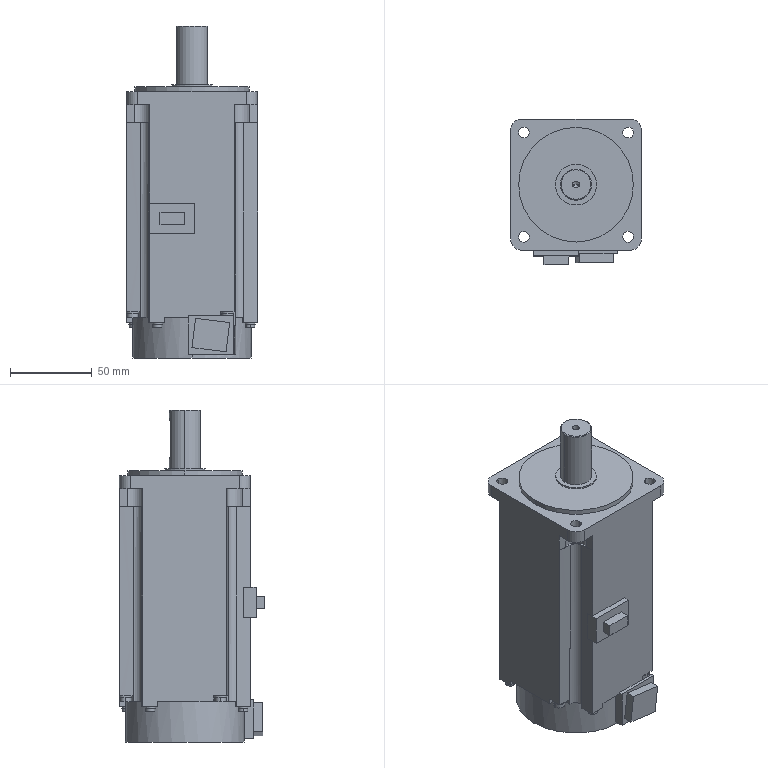Part | STEP file | Servo motor HG-KN73BJK-S100 750w_with brake_with keyway_Mitsubishi | 1 solid | 187 faces | box 80.44 x 89.02 x 202.7 mm | volume 918886 mm3 | plane 98 | cylinder 85 | cone 4 | commonest cylinder face diameters 920 x16 5.5 x8 5.9 x8 6.6 x8 7 x8 7.6 x8